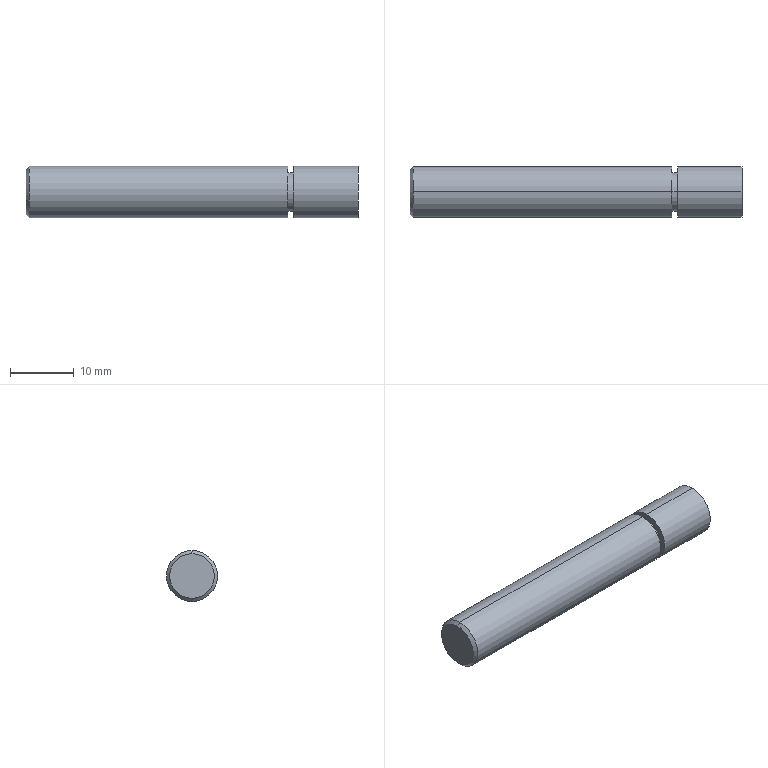Part | STEP file | 0246_222_Pin | 1 solid | 15 faces | box 52 x 8 x 8 mm | volume 2505 mm3 | cylinder 8 | plane 5 | cone 2 | commonest cylinder face diameters 8 x4 3.3 x2 6 x2
STEP:
#1=CARTESIAN_POINT('',(0.,0.,0.));
#2=DIRECTION('',(0.,0.,1.));
#3=DIRECTION('',(1.,0.,0.));
#4=AXIS2_PLACEMENT_3D('',#1,#2,#3);
#5=CARTESIAN_POINT('',(-41.,0.,3.5));
#6=VERTEX_POINT('',#5);
#7=CARTESIAN_POINT('',(-41.,0.,-3.5));
#8=VERTEX_POINT('',#7);
#9=CARTESIAN_POINT('',(-41.,0.,0.));
#10=DIRECTION('',(-1.,0.,0.));
#11=DIRECTION('',(0.,0.,-1.));
#12=AXIS2_PLACEMENT_3D('',#9,#10,#11);
#13=CIRCLE('',#12,3.5);
#14=CARTESIAN_POINT('',(-41.,0.,0.));
#15=DIRECTION('',(1.,0.,0.));
#16=DIRECTION('',(0.,0.,-1.));
#17=AXIS2_PLACEMENT_3D('',#14,#15,#16);
#18=CONICAL_SURFACE('',#17,3.5,0.7854);
#19=CARTESIAN_POINT('',(6.283,0.));
#20=DIRECTION('',(-1.,0.));
#21=VECTOR('',#20,1.);
#22=LINE('',#19,#21);
#23=(GEOMETRIC_REPRESENTATION_CONTEXT(2)PARAMETRIC_REPRESENTATION_CONTEXT()REPRESENTATION_CONTEXT('',''));
#24=DEFINITIONAL_REPRESENTATION('',(#22),#23);
#25=PCURVE('',#18,#24);
#26=CARTESIAN_POINT('',(-41.,-4.,0.));
#27=DIRECTION('',(1.,0.,0.));
#28=DIRECTION('',(0.,0.,-1.));
#29=AXIS2_PLACEMENT_3D('',#26,#27,#28);
#30=PLANE('',#29);
#31=CARTESIAN_POINT('',(3.5,4.));
#32=CARTESIAN_POINT('',(3.5,-2.062));
#33=CARTESIAN_POINT('',(-1.75,0.9689));
#34=CARTESIAN_POINT('',(-7.,4.));
#35=CARTESIAN_POINT('',(-1.75,7.031));
#36=CARTESIAN_POINT('',(3.5,10.062));
#37=CARTESIAN_POINT('',(3.5,4.));
#38=(BOUNDED_CURVE()B_SPLINE_CURVE(2,(#31,#32,#33,#34,#35,#36,#37),.UNSPECIFIED.,.T.,.F.)B_SPLINE_CURVE_WITH_KNOTS((1,2,2,2,2,1),(-2.094,0.,2.094,4.189,6.283,8.378),.UNSPECIFIED.)CURVE()GEOMETRIC_REPRESENTATION_ITEM()RATIONAL_B_SPLINE_CURVE((1.,0.5,1.,0.5,1.,0.5,1.))REPRESENTATION_ITEM(''));
#39=(GEOMETRIC_REPRESENTATION_CONTEXT(2)PARAMETRIC_REPRESENTATION_CONTEXT()REPRESENTATION_CONTEXT('',''));
#40=DEFINITIONAL_REPRESENTATION('',(#38),#39);
#41=PCURVE('',#30,#40);
#42=SURFACE_CURVE('',#13,(#25,#41),.PCURVE_S1.);
#43=EDGE_CURVE('',#6,#8,#42,.T.);
#44=ORIENTED_EDGE('',*,*,#43,.F.);
#45=CARTESIAN_POINT('',(-40.5,0.,4.));
#46=VERTEX_POINT('',#45);
#47=CARTESIAN_POINT('',(-41.,0.,3.5));
#48=DIRECTION('',(0.7071,0.,0.7071));
#49=VECTOR('',#48,1.);
#50=LINE('',#47,#49);
#51=CARTESIAN_POINT('',(3.142,0.));
#52=DIRECTION('',(0.,1.));
#53=VECTOR('',#52,1.);
#54=LINE('',#51,#53);
#55=(GEOMETRIC_REPRESENTATION_CONTEXT(2)PARAMETRIC_REPRESENTATION_CONTEXT()REPRESENTATION_CONTEXT('',''));
#56=DEFINITIONAL_REPRESENTATION('',(#54),#55);
#57=PCURVE('',#18,#56);
#58=CARTESIAN_POINT('',(-41.,0.,0.));
#59=DIRECTION('',(1.,0.,0.));
#60=DIRECTION('',(0.,0.,-1.));
#61=AXIS2_PLACEMENT_3D('',#58,#59,#60);
#62=CONICAL_SURFACE('',#61,3.5,0.7854);
#63=CARTESIAN_POINT('',(3.142,0.));
#64=DIRECTION('',(0.,1.));
#65=VECTOR('',#64,1.);
#66=LINE('',#63,#65);
#67=(GEOMETRIC_REPRESENTATION_CONTEXT(2)PARAMETRIC_REPRESENTATION_CONTEXT()REPRESENTATION_CONTEXT('',''));
#68=DEFINITIONAL_REPRESENTATION('',(#66),#67);
#69=PCURVE('',#62,#68);
#70=SURFACE_CURVE('',#50,(#57,#69),.PCURVE_S1.);
#71=EDGE_CURVE('',#6,#46,#70,.T.);
#72=ORIENTED_EDGE('',*,*,#71,.T.);
#73=CARTESIAN_POINT('',(-40.5,0.,-4.));
#74=VERTEX_POINT('',#73);
#75=CARTESIAN_POINT('',(-40.5,0.,0.));
#76=DIRECTION('',(1.,0.,0.));
#77=DIRECTION('',(0.,0.,-1.));
#78=AXIS2_PLACEMENT_3D('',#75,#76,#77);
#79=CIRCLE('',#78,4.);
#80=CARTESIAN_POINT('',(0.,0.5));
#81=DIRECTION('',(1.,0.));
#82=VECTOR('',#81,1.);
#83=LINE('',#80,#82);
#84=(GEOMETRIC_REPRESENTATION_CONTEXT(2)PARAMETRIC_REPRESENTATION_CONTEXT()REPRESENTATION_CONTEXT('',''));
#85=DEFINITIONAL_REPRESENTATION('',(#83),#84);
#86=PCURVE('',#18,#85);
#87=CARTESIAN_POINT('',(-41.,0.,0.));
#88=DIRECTION('',(-1.,0.,0.));
#89=DIRECTION('',(0.,0.,1.));
#90=AXIS2_PLACEMENT_3D('',#87,#88,#89);
#91=CYLINDRICAL_SURFACE('',#90,4.);
#92=CARTESIAN_POINT('',(3.142,-0.5));
#93=DIRECTION('',(-1.,0.));
#94=VECTOR('',#93,1.);
#95=LINE('',#92,#94);
#96=(GEOMETRIC_REPRESENTATION_CONTEXT(2)PARAMETRIC_REPRESENTATION_CONTEXT()REPRESENTATION_CONTEXT('',''));
#97=DEFINITIONAL_REPRESENTATION('',(#95),#96);
#98=PCURVE('',#91,#97);
#99=SURFACE_CURVE('',#79,(#86,#98),.PCURVE_S1.);
#100=EDGE_CURVE('',#74,#46,#99,.T.);
#101=ORIENTED_EDGE('',*,*,#100,.F.);
#102=CARTESIAN_POINT('',(-41.,0.,-3.5));
#103=DIRECTION('',(0.7071,0.,-0.7071));
#104=VECTOR('',#103,1.);
#105=LINE('',#102,#104);
#106=CARTESIAN_POINT('',(0.,0.));
#107=DIRECTION('',(0.,1.));
#108=VECTOR('',#107,1.);
#109=LINE('',#106,#108);
#110=(GEOMETRIC_REPRESENTATION_CONTEXT(2)PARAMETRIC_REPRESENTATION_CONTEXT()REPRESENTATION_CONTEXT('',''));
#111=DEFINITIONAL_REPRESENTATION('',(#109),#110);
#112=PCURVE('',#18,#111);
#113=CARTESIAN_POINT('',(6.283,0.));
#114=DIRECTION('',(0.,1.));
#115=VECTOR('',#114,1.);
#116=LINE('',#113,#115);
#117=(GEOMETRIC_REPRESENTATION_CONTEXT(2)PARAMETRIC_REPRESENTATION_CONTEXT()REPRESENTATION_CONTEXT('',''));
#118=DEFINITIONAL_REPRESENTATION('',(#116),#117);
#119=PCURVE('',#62,#118);
#120=SURFACE_CURVE('',#105,(#112,#119),.PCURVE_S1.);
#121=EDGE_CURVE('',#8,#74,#120,.T.);
#122=ORIENTED_EDGE('',*,*,#121,.F.);
#123=EDGE_LOOP('',(#44,#72,#101,#122));
#124=FACE_BOUND('',#123,.T.);
#125=ADVANCED_FACE('',(#124),#18,.T.);
#126=CARTESIAN_POINT('',(0.9,0.,-1.65));
#127=VERTEX_POINT('',#126);
#128=CARTESIAN_POINT('',(11.,0.,-1.65));
#129=VERTEX_POINT('',#128);
#130=CARTESIAN_POINT('',(11.,0.,-1.65));
#131=DIRECTION('',(1.,0.,0.));
#132=VECTOR('',#131,1.);
#133=LINE('',#130,#132);
#134=CARTESIAN_POINT('',(11.,0.,0.));
#135=DIRECTION('',(1.,0.,0.));
#136=DIRECTION('',(0.,0.,-1.));
#137=AXIS2_PLACEMENT_3D('',#134,#135,#136);
#138=CYLINDRICAL_SURFACE('',#137,1.65);
#139=CARTESIAN_POINT('',(6.283,0.));
#140=DIRECTION('',(0.,1.));
#141=VECTOR('',#140,1.);
#142=LINE('',#139,#141);
#143=(GEOMETRIC_REPRESENTATION_CONTEXT(2)PARAMETRIC_REPRESENTATION_CONTEXT()REPRESENTATION_CONTEXT('',''));
#144=DEFINITIONAL_REPRESENTATION('',(#142),#143);
#145=PCURVE('',#138,#144);
#146=CARTESIAN_POINT('',(11.,0.,0.));
#147=DIRECTION('',(1.,0.,0.));
#148=DIRECTION('',(0.,0.,-1.));
#149=AXIS2_PLACEMENT_3D('',#146,#147,#148);
#150=CYLINDRICAL_SURFACE('',#149,1.65);
#151=CARTESIAN_POINT('',(0.,0.));
#152=DIRECTION('',(0.,1.));
#153=VECTOR('',#152,1.);
#154=LINE('',#151,#153);
#155=(GEOMETRIC_REPRESENTATION_CONTEXT(2)PARAMETRIC_REPRESENTATION_CONTEXT()REPRESENTATION_CONTEXT('',''));
#156=DEFINITIONAL_REPRESENTATION('',(#154),#155);
#157=PCURVE('',#150,#156);
#158=SURFACE_CURVE('',#133,(#145,#157),.PCURVE_S1.);
#159=EDGE_CURVE('',#127,#129,#158,.T.);
#160=ORIENTED_EDGE('',*,*,#159,.T.);
#161=CARTESIAN_POINT('',(11.,0.,1.65));
#162=VERTEX_POINT('',#161);
#163=CARTESIAN_POINT('',(11.,0.,0.));
#164=DIRECTION('',(1.,0.,0.));
#165=DIRECTION('',(0.,0.,-1.));
#166=AXIS2_PLACEMENT_3D('',#163,#164,#165);
#167=CIRCLE('',#166,1.65);
#168=CARTESIAN_POINT('',(0.,0.));
#169=DIRECTION('',(1.,0.));
#170=VECTOR('',#169,1.);
#171=LINE('',#168,#170);
#172=(GEOMETRIC_REPRESENTATION_CONTEXT(2)PARAMETRIC_REPRESENTATION_CONTEXT()REPRESENTATION_CONTEXT('',''));
#173=DEFINITIONAL_REPRESENTATION('',(#171),#172);
#174=PCURVE('',#138,#173);
#175=CARTESIAN_POINT('',(11.,-4.,0.));
#176=DIRECTION('',(-1.,0.,0.));
#177=DIRECTION('',(0.,0.,1.));
#178=AXIS2_PLACEMENT_3D('',#175,#176,#177);
#179=PLANE('',#178);
#180=CARTESIAN_POINT('',(-1.65,4.));
#181=CARTESIAN_POINT('',(-1.65,6.858));
#182=CARTESIAN_POINT('',(0.825,5.429));
#183=CARTESIAN_POINT('',(3.3,4.));
#184=CARTESIAN_POINT('',(0.825,2.571));
#185=CARTESIAN_POINT('',(-1.65,1.142));
#186=CARTESIAN_POINT('',(-1.65,4.));
#187=(BOUNDED_CURVE()B_SPLINE_CURVE(2,(#180,#181,#182,#183,#184,#185,#186),.UNSPECIFIED.,.T.,.F.)B_SPLINE_CURVE_WITH_KNOTS((1,2,2,2,2,1),(-2.094,0.,2.094,4.189,6.283,8.378),.UNSPECIFIED.)CURVE()GEOMETRIC_REPRESENTATION_ITEM()RATIONAL_B_SPLINE_CURVE((1.,0.5,1.,0.5,1.,0.5,1.))REPRESENTATION_ITEM(''));
#188=(GEOMETRIC_REPRESENTATION_CONTEXT(2)PARAMETRIC_REPRESENTATION_CONTEXT()REPRESENTATION_CONTEXT('',''));
#189=DEFINITIONAL_REPRESENTATION('',(#187),#188);
#190=PCURVE('',#179,#189);
#191=SURFACE_CURVE('',#167,(#174,#190),.PCURVE_S1.);
#192=EDGE_CURVE('',#162,#129,#191,.T.);
#193=ORIENTED_EDGE('',*,*,#192,.F.);
#194=CARTESIAN_POINT('',(0.9,0.,1.65));
#195=VERTEX_POINT('',#194);
#196=CARTESIAN_POINT('',(11.,0.,1.65));
#197=DIRECTION('',(1.,0.,0.));
#198=VECTOR('',#197,1.);
#199=LINE('',#196,#198);
#200=CARTESIAN_POINT('',(3.142,0.));
#201=DIRECTION('',(0.,1.));
#202=VECTOR('',#201,1.);
#203=LINE('',#200,#202);
#204=(GEOMETRIC_REPRESENTATION_CONTEXT(2)PARAMETRIC_REPRESENTATION_CONTEXT()REPRESENTATION_CONTEXT('',''));
#205=DEFINITIONAL_REPRESENTATION('',(#203),#204);
#206=PCURVE('',#138,#205);
#207=CARTESIAN_POINT('',(3.142,0.));
#208=DIRECTION('',(0.,1.));
#209=VECTOR('',#208,1.);
#210=LINE('',#207,#209);
#211=(GEOMETRIC_REPRESENTATION_CONTEXT(2)PARAMETRIC_REPRESENTATION_CONTEXT()REPRESENTATION_CONTEXT('',''));
#212=DEFINITIONAL_REPRESENTATION('',(#210),#211);
#213=PCURVE('',#150,#212);
#214=SURFACE_CURVE('',#199,(#206,#213),.PCURVE_S1.);
#215=EDGE_CURVE('',#195,#162,#214,.T.);
#216=ORIENTED_EDGE('',*,*,#215,.F.);
#217=CARTESIAN_POINT('',(0.9,0.,0.));
#218=DIRECTION('',(1.,0.,0.));
#219=DIRECTION('',(0.,0.,-1.));
#220=AXIS2_PLACEMENT_3D('',#217,#218,#219);
#221=CIRCLE('',#220,1.65);
#222=CARTESIAN_POINT('',(0.,-10.1));
#223=DIRECTION('',(1.,0.));
#224=VECTOR('',#223,1.);
#225=LINE('',#222,#224);
#226=(GEOMETRIC_REPRESENTATION_CONTEXT(2)PARAMETRIC_REPRESENTATION_CONTEXT()REPRESENTATION_CONTEXT('',''));
#227=DEFINITIONAL_REPRESENTATION('',(#225),#226);
#228=PCURVE('',#138,#227);
#229=CARTESIAN_POINT('',(0.9,0.,0.));
#230=DIRECTION('',(-1.,0.,0.));
#231=DIRECTION('',(0.,0.,1.));
#232=AXIS2_PLACEMENT_3D('',#229,#230,#231);
#233=PLANE('',#232);
#234=CARTESIAN_POINT('',(-1.65,0.));
#235=CARTESIAN_POINT('',(-1.65,2.858));
#236=CARTESIAN_POINT('',(0.825,1.429));
#237=CARTESIAN_POINT('',(3.3,0.));
#238=CARTESIAN_POINT('',(0.825,-1.429));
#239=CARTESIAN_POINT('',(-1.65,-2.858));
#240=CARTESIAN_POINT('',(-1.65,0.));
#241=(BOUNDED_CURVE()B_SPLINE_CURVE(2,(#234,#235,#236,#237,#238,#239,#240),.UNSPECIFIED.,.T.,.F.)B_SPLINE_CURVE_WITH_KNOTS((1,2,2,2,2,1),(-2.094,0.,2.094,4.189,6.283,8.378),.UNSPECIFIED.)CURVE()GEOMETRIC_REPRESENTATION_ITEM()RATIONAL_B_SPLINE_CURVE((1.,0.5,1.,0.5,1.,0.5,1.))REPRESENTATION_ITEM(''));
#242=(GEOMETRIC_REPRESENTATION_CONTEXT(2)PARAMETRIC_REPRESENTATION_CONTEXT()REPRESENTATION_CONTEXT('',''));
#243=DEFINITIONAL_REPRESENTATION('',(#241),#242);
#244=PCURVE('',#233,#243);
#245=SURFACE_CURVE('',#221,(#228,#244),.PCURVE_S1.);
#246=EDGE_CURVE('',#195,#127,#245,.T.);
#247=ORIENTED_EDGE('',*,*,#246,.T.);
#248=EDGE_LOOP('',(#160,#193,#216,#247));
#249=FACE_BOUND('',#248,.F.);
#250=ADVANCED_FACE('',(#249),#138,.F.);
#251=CARTESIAN_POINT('',(11.,0.,4.));
#252=VERTEX_POINT('',#251);
#253=CARTESIAN_POINT('',(11.,0.,-4.));
#254=VERTEX_POINT('',#253);
#255=CARTESIAN_POINT('',(11.,0.,0.));
#256=DIRECTION('',(-1.,0.,0.));
#257=DIRECTION('',(0.,0.,1.));
#258=AXIS2_PLACEMENT_3D('',#255,#256,#257);
#259=CIRCLE('',#258,4.);
#260=CARTESIAN_POINT('',(-41.,0.,0.));
#261=DIRECTION('',(-1.,0.,0.));
#262=DIRECTION('',(0.,0.,1.));
#263=AXIS2_PLACEMENT_3D('',#260,#261,#262);
#264=CYLINDRICAL_SURFACE('',#263,4.);
#265=CARTESIAN_POINT('',(0.,-52.));
#266=DIRECTION('',(1.,0.));
#267=VECTOR('',#266,1.);
#268=LINE('',#265,#267);
#269=(GEOMETRIC_REPRESENTATION_CONTEXT(2)PARAMETRIC_REPRESENTATION_CONTEXT()REPRESENTATION_CONTEXT('',''));
#270=DEFINITIONAL_REPRESENTATION('',(#268),#269);
#271=PCURVE('',#264,#270);
#272=CARTESIAN_POINT('',(0.,4.));
#273=DIRECTION('',(1.,0.));
#274=AXIS2_PLACEMENT_2D('',#272,#273);
#275=CIRCLE('',#274,4.);
#276=(GEOMETRIC_REPRESENTATION_CONTEXT(2)PARAMETRIC_REPRESENTATION_CONTEXT()REPRESENTATION_CONTEXT('',''));
#277=DEFINITIONAL_REPRESENTATION('',(#275),#276);
#278=PCURVE('',#179,#277);
#279=SURFACE_CURVE('',#259,(#271,#278),.PCURVE_S1.);
#280=EDGE_CURVE('',#252,#254,#279,.T.);
#281=ORIENTED_EDGE('',*,*,#280,.T.);
#282=CARTESIAN_POINT('',(0.9,0.,-4.));
#283=VERTEX_POINT('',#282);
#284=CARTESIAN_POINT('',(-41.,0.,-4.));
#285=DIRECTION('',(-1.,0.,0.));
#286=VECTOR('',#285,1.);
#287=LINE('',#284,#286);
#288=CARTESIAN_POINT('',(3.142,0.));
#289=DIRECTION('',(0.,1.));
#290=VECTOR('',#289,1.);
#291=LINE('',#288,#290);
#292=(GEOMETRIC_REPRESENTATION_CONTEXT(2)PARAMETRIC_REPRESENTATION_CONTEXT()REPRESENTATION_CONTEXT('',''));
#293=DEFINITIONAL_REPRESENTATION('',(#291),#292);
#294=PCURVE('',#264,#293);
#295=CARTESIAN_POINT('',(-41.,0.,0.));
#296=DIRECTION('',(-1.,0.,0.));
#297=DIRECTION('',(0.,0.,1.));
#298=AXIS2_PLACEMENT_3D('',#295,#296,#297);
#299=CYLINDRICAL_SURFACE('',#298,4.);
#300=CARTESIAN_POINT('',(3.142,0.));
#301=DIRECTION('',(0.,1.));
#302=VECTOR('',#301,1.);
#303=LINE('',#300,#302);
#304=(GEOMETRIC_REPRESENTATION_CONTEXT(2)PARAMETRIC_REPRESENTATION_CONTEXT()REPRESENTATION_CONTEXT('',''));
#305=DEFINITIONAL_REPRESENTATION('',(#303),#304);
#306=PCURVE('',#299,#305);
#307=SURFACE_CURVE('',#287,(#294,#306),.PCURVE_S1.);
#308=EDGE_CURVE('',#254,#283,#307,.T.);
#309=ORIENTED_EDGE('',*,*,#308,.T.);
#310=CARTESIAN_POINT('',(0.9,0.,4.));
#311=VERTEX_POINT('',#310);
#312=CARTESIAN_POINT('',(0.9,0.,0.));
#313=DIRECTION('',(-1.,0.,0.));
#314=DIRECTION('',(0.,0.,1.));
#315=AXIS2_PLACEMENT_3D('',#312,#313,#314);
#316=CIRCLE('',#315,4.);
#317=CARTESIAN_POINT('',(0.,-41.9));
#318=DIRECTION('',(1.,0.));
#319=VECTOR('',#318,1.);
#320=LINE('',#317,#319);
#321=(GEOMETRIC_REPRESENTATION_CONTEXT(2)PARAMETRIC_REPRESENTATION_CONTEXT()REPRESENTATION_CONTEXT('',''));
#322=DEFINITIONAL_REPRESENTATION('',(#320),#321);
#323=PCURVE('',#264,#322);
#324=CARTESIAN_POINT('',(0.9,-3.,0.));
#325=DIRECTION('',(1.,0.,0.));
#326=DIRECTION('',(0.,0.,-1.));
#327=AXIS2_PLACEMENT_3D('',#324,#325,#326);
#328=PLANE('',#327);
#329=CARTESIAN_POINT('',(-4.,3.));
#330=CARTESIAN_POINT('',(-4.,9.928));
#331=CARTESIAN_POINT('',(2.,6.464));
#332=CARTESIAN_POINT('',(8.,3.));
#333=CARTESIAN_POINT('',(2.,-0.4641));
#334=CARTESIAN_POINT('',(-4.,-3.928));
#335=CARTESIAN_POINT('',(-4.,3.));
#336=(BOUNDED_CURVE()B_SPLINE_CURVE(2,(#329,#330,#331,#332,#333,#334,#335),.UNSPECIFIED.,.T.,.F.)B_SPLINE_CURVE_WITH_KNOTS((1,2,2,2,2,1),(-2.094,0.,2.094,4.189,6.283,8.378),.UNSPECIFIED.)CURVE()GEOMETRIC_REPRESENTATION_ITEM()RATIONAL_B_SPLINE_CURVE((1.,0.5,1.,0.5,1.,0.5,1.))REPRESENTATION_ITEM(''));
#337=(GEOMETRIC_REPRESENTATION_CONTEXT(2)PARAMETRIC_REPRESENTATION_CONTEXT()REPRESENTATION_CONTEXT('',''));
#338=DEFINITIONAL_REPRESENTATION('',(#336),#337);
#339=PCURVE('',#328,#338);
#340=SURFACE_CURVE('',#316,(#323,#339),.PCURVE_S1.);
#341=EDGE_CURVE('',#311,#283,#340,.T.);
#342=ORIENTED_EDGE('',*,*,#341,.F.);
#343=CARTESIAN_POINT('',(-41.,0.,4.));
#344=DIRECTION('',(-1.,0.,0.));
#345=VECTOR('',#344,1.);
#346=LINE('',#343,#345);
#347=CARTESIAN_POINT('',(0.,0.));
#348=DIRECTION('',(0.,1.));
#349=VECTOR('',#348,1.);
#350=LINE('',#347,#349);
#351=(GEOMETRIC_REPRESENTATION_CONTEXT(2)PARAMETRIC_REPRESENTATION_CONTEXT()REPRESENTATION_CONTEXT('',''));
#352=DEFINITIONAL_REPRESENTATION('',(#350),#351);
#353=PCURVE('',#264,#352);
#354=CARTESIAN_POINT('',(6.283,0.));
#355=DIRECTION('',(0.,1.));
#356=VECTOR('',#355,1.);
#357=LINE('',#354,#356);
#358=(GEOMETRIC_REPRESENTATION_CONTEXT(2)PARAMETRIC_REPRESENTATION_CONTEXT()REPRESENTATION_CONTEXT('',''));
#359=DEFINITIONAL_REPRESENTATION('',(#357),#358);
#360=PCURVE('',#299,#359);
#361=SURFACE_CURVE('',#346,(#353,#360),.PCURVE_S1.);
#362=EDGE_CURVE('',#252,#311,#361,.T.);
#363=ORIENTED_EDGE('',*,*,#362,.F.);
#364=EDGE_LOOP('',(#281,#309,#342,#363));
#365=FACE_BOUND('',#364,.T.);
#366=ADVANCED_FACE('',(#365),#264,.T.);
#367=CARTESIAN_POINT('',(0.9,0.,3.));
#368=VERTEX_POINT('',#367);
#369=CARTESIAN_POINT('',(0.9,0.,-3.));
#370=VERTEX_POINT('',#369);
#371=CARTESIAN_POINT('',(0.9,0.,0.));
#372=DIRECTION('',(-1.,0.,0.));
#373=DIRECTION('',(0.,0.,1.));
#374=AXIS2_PLACEMENT_3D('',#371,#372,#373);
#375=CIRCLE('',#374,3.);
#376=CARTESIAN_POINT('',(-41.,0.,0.));
#377=DIRECTION('',(-1.,0.,0.));
#378=DIRECTION('',(0.,0.,1.));
#379=AXIS2_PLACEMENT_3D('',#376,#377,#378);
#380=CYLINDRICAL_SURFACE('',#379,3.);
#381=CARTESIAN_POINT('',(0.,-41.9));
#382=DIRECTION('',(1.,0.));
#383=VECTOR('',#382,1.);
#384=LINE('',#381,#383);
#385=(GEOMETRIC_REPRESENTATION_CONTEXT(2)PARAMETRIC_REPRESENTATION_CONTEXT()REPRESENTATION_CONTEXT('',''));
#386=DEFINITIONAL_REPRESENTATION('',(#384),#385);
#387=PCURVE('',#380,#386);
#388=CARTESIAN_POINT('',(-3.,3.));
#389=CARTESIAN_POINT('',(-3.,8.196));
#390=CARTESIAN_POINT('',(1.5,5.598));
#391=CARTESIAN_POINT('',(6.,3.));
#392=CARTESIAN_POINT('',(1.5,0.4019));
#393=CARTESIAN_POINT('',(-3.,-2.196));
#394=CARTESIAN_POINT('',(-3.,3.));
#395=(BOUNDED_CURVE()B_SPLINE_CURVE(2,(#388,#389,#390,#391,#392,#393,#394),.UNSPECIFIED.,.T.,.F.)B_SPLINE_CURVE_WITH_KNOTS((1,2,2,2,2,1),(-2.094,0.,2.094,4.189,6.283,8.378),.UNSPECIFIED.)CURVE()GEOMETRIC_REPRESENTATION_ITEM()RATIONAL_B_SPLINE_CURVE((1.,0.5,1.,0.5,1.,0.5,1.))REPRESENTATION_ITEM(''));
#396=(GEOMETRIC_REPRESENTATION_CONTEXT(2)PARAMETRIC_REPRESENTATION_CONTEXT()REPRESENTATION_CONTEXT('',''));
#397=DEFINITIONAL_REPRESENTATION('',(#395),#396);
#398=PCURVE('',#328,#397);
#399=SURFACE_CURVE('',#375,(#387,#398),.PCURVE_S1.);
#400=EDGE_CURVE('',#368,#370,#399,.T.);
#401=ORIENTED_EDGE('',*,*,#400,.T.);
#402=CARTESIAN_POINT('',(0.,0.,-3.));
#403=VERTEX_POINT('',#402);
#404=CARTESIAN_POINT('',(-41.,0.,-3.));
#405=DIRECTION('',(-1.,0.,0.));
#406=VECTOR('',#405,1.);
#407=LINE('',#404,#406);
#408=CARTESIAN_POINT('',(3.142,0.));
#409=DIRECTION('',(0.,1.));
#410=VECTOR('',#409,1.);
#411=LINE('',#408,#410);
#412=(GEOMETRIC_REPRESENTATION_CONTEXT(2)PARAMETRIC_REPRESENTATION_CONTEXT()REPRESENTATION_CONTEXT('',''));
#413=DEFINITIONAL_REPRESENTATION('',(#411),#412);
#414=PCURVE('',#380,#413);
#415=CARTESIAN_POINT('',(-41.,0.,0.));
#416=DIRECTION('',(-1.,0.,0.));
#417=DIRECTION('',(0.,0.,1.));
#418=AXIS2_PLACEMENT_3D('',#415,#416,#417);
#419=CYLINDRICAL_SURFACE('',#418,3.);
#420=CARTESIAN_POINT('',(3.142,0.));
#421=DIRECTION('',(0.,1.));
#422=VECTOR('',#421,1.);
#423=LINE('',#420,#422);
#424=(GEOMETRIC_REPRESENTATION_CONTEXT(2)PARAMETRIC_REPRESENTATION_CONTEXT()REPRESENTATION_CONTEXT('',''));
#425=DEFINITIONAL_REPRESENTATION('',(#423),#424);
#426=PCURVE('',#419,#425);
#427=SURFACE_CURVE('',#407,(#414,#426),.PCURVE_S1.);
#428=EDGE_CURVE('',#370,#403,#427,.T.);
#429=ORIENTED_EDGE('',*,*,#428,.T.);
#430=CARTESIAN_POINT('',(0.,0.,3.));
#431=VERTEX_POINT('',#430);
#432=CARTESIAN_POINT('',(0.,0.,0.));
#433=DIRECTION('',(-1.,0.,0.));
#434=DIRECTION('',(0.,0.,1.));
#435=AXIS2_PLACEMENT_3D('',#432,#433,#434);
#436=CIRCLE('',#435,3.);
#437=CARTESIAN_POINT('',(0.,-41.));
#438=DIRECTION('',(1.,0.));
#439=VECTOR('',#438,1.);
#440=LINE('',#437,#439);
#441=(GEOMETRIC_REPRESENTATION_CONTEXT(2)PARAMETRIC_REPRESENTATION_CONTEXT()REPRESENTATION_CONTEXT('',''));
#442=DEFINITIONAL_REPRESENTATION('',(#440),#441);
#443=PCURVE('',#380,#442);
#444=CARTESIAN_POINT('',(0.,-3.,0.));
#445=DIRECTION('',(-1.,0.,0.));
#446=DIRECTION('',(0.,0.,1.));
#447=AXIS2_PLACEMENT_3D('',#444,#445,#446);
#448=PLANE('',#447);
#449=CARTESIAN_POINT('',(0.,3.));
#450=DIRECTION('',(1.,0.));
#451=AXIS2_PLACEMENT_2D('',#449,#450);
#452=CIRCLE('',#451,3.);
#453=(GEOMETRIC_REPRESENTATION_CONTEXT(2)PARAMETRIC_REPRESENTATION_CONTEXT()REPRESENTATION_CONTEXT('',''));
#454=DEFINITIONAL_REPRESENTATION('',(#452),#453);
#455=PCURVE('',#448,#454);
#456=SURFACE_CURVE('',#436,(#443,#455),.PCURVE_S1.);
#457=EDGE_CURVE('',#431,#403,#456,.T.);
#458=ORIENTED_EDGE('',*,*,#457,.F.);
#459=CARTESIAN_POINT('',(-41.,0.,3.));
#460=DIRECTION('',(-1.,0.,0.));
#461=VECTOR('',#460,1.);
#462=LINE('',#459,#461);
#463=CARTESIAN_POINT('',(0.,0.));
#464=DIRECTION('',(0.,1.));
#465=VECTOR('',#464,1.);
#466=LINE('',#463,#465);
#467=(GEOMETRIC_REPRESENTATION_CONTEXT(2)PARAMETRIC_REPRESENTATION_CONTEXT()REPRESENTATION_CONTEXT('',''));
#468=DEFINITIONAL_REPRESENTATION('',(#466),#467);
#469=PCURVE('',#380,#468);
#470=CARTESIAN_POINT('',(6.283,0.));
#471=DIRECTION('',(0.,1.));
#472=VECTOR('',#471,1.);
#473=LINE('',#470,#472);
#474=(GEOMETRIC_REPRESENTATION_CONTEXT(2)PARAMETRIC_REPRESENTATION_CONTEXT()REPRESENTATION_CONTEXT('',''));
#475=DEFINITIONAL_REPRESENTATION('',(#473),#474);
#476=PCURVE('',#419,#475);
#477=SURFACE_CURVE('',#462,(#469,#476),.PCURVE_S1.);
#478=EDGE_CURVE('',#368,#431,#477,.T.);
#479=ORIENTED_EDGE('',*,*,#478,.F.);
#480=EDGE_LOOP('',(#401,#429,#458,#479));
#481=FACE_BOUND('',#480,.T.);
#482=ADVANCED_FACE('',(#481),#380,.T.);
#483=CARTESIAN_POINT('',(0.,0.,4.));
#484=VERTEX_POINT('',#483);
#485=CARTESIAN_POINT('',(0.,0.,-4.));
#486=VERTEX_POINT('',#485);
#487=CARTESIAN_POINT('',(0.,0.,0.));
#488=DIRECTION('',(-1.,0.,0.));
#489=DIRECTION('',(0.,0.,1.));
#490=AXIS2_PLACEMENT_3D('',#487,#488,#489);
#491=CIRCLE('',#490,4.);
#492=CARTESIAN_POINT('',(0.,-41.));
#493=DIRECTION('',(1.,0.));
#494=VECTOR('',#493,1.);
#495=LINE('',#492,#494);
#496=(GEOMETRIC_REPRESENTATION_CONTEXT(2)PARAMETRIC_REPRESENTATION_CONTEXT()REPRESENTATION_CONTEXT('',''));
#497=DEFINITIONAL_REPRESENTATION('',(#495),#496);
#498=PCURVE('',#91,#497);
#499=CARTESIAN_POINT('',(0.,3.));
#500=DIRECTION('',(1.,0.));
#501=AXIS2_PLACEMENT_2D('',#499,#500);
#502=CIRCLE('',#501,4.);
#503=(GEOMETRIC_REPRESENTATION_CONTEXT(2)PARAMETRIC_REPRESENTATION_CONTEXT()REPRESENTATION_CONTEXT('',''));
#504=DEFINITIONAL_REPRESENTATION('',(#502),#503);
#505=PCURVE('',#448,#504);
#506=SURFACE_CURVE('',#491,(#498,#505),.PCURVE_S1.);
#507=EDGE_CURVE('',#484,#486,#506,.T.);
#508=ORIENTED_EDGE('',*,*,#507,.T.);
#509=CARTESIAN_POINT('',(-41.,0.,-4.));
#510=DIRECTION('',(-1.,0.,0.));
#511=VECTOR('',#510,1.);
#512=LINE('',#509,#511);
#513=CARTESIAN_POINT('',(3.142,0.));
#514=DIRECTION('',(0.,1.));
#515=VECTOR('',#514,1.);
#516=LINE('',#513,#515);
#517=(GEOMETRIC_REPRESENTATION_CONTEXT(2)PARAMETRIC_REPRESENTATION_CONTEXT()REPRESENTATION_CONTEXT('',''));
#518=DEFINITIONAL_REPRESENTATION('',(#516),#517);
#519=PCURVE('',#91,#518);
#520=CARTESIAN_POINT('',(-41.,0.,0.));
#521=DIRECTION('',(-1.,0.,0.));
#522=DIRECTION('',(0.,0.,1.));
#523=AXIS2_PLACEMENT_3D('',#520,#521,#522);
#524=CYLINDRICAL_SURFACE('',#523,4.);
#525=CARTESIAN_POINT('',(3.142,0.));
#526=DIRECTION('',(0.,1.));
#527=VECTOR('',#526,1.);
#528=LINE('',#525,#527);
#529=(GEOMETRIC_REPRESENTATION_CONTEXT(2)PARAMETRIC_REPRESENTATION_CONTEXT()REPRESENTATION_CONTEXT('',''));
#530=DEFINITIONAL_REPRESENTATION('',(#528),#529);
#531=PCURVE('',#524,#530);
#532=SURFACE_CURVE('',#512,(#519,#531),.PCURVE_S1.);
#533=EDGE_CURVE('',#486,#74,#532,.T.);
#534=ORIENTED_EDGE('',*,*,#533,.T.);
#535=ORIENTED_EDGE('',*,*,#100,.T.);
#536=CARTESIAN_POINT('',(-41.,0.,4.));
#537=DIRECTION('',(-1.,0.,0.));
#538=VECTOR('',#537,1.);
#539=LINE('',#536,#538);
#540=CARTESIAN_POINT('',(0.,0.));
#541=DIRECTION('',(0.,1.));
#542=VECTOR('',#541,1.);
#543=LINE('',#540,#542);
#544=(GEOMETRIC_REPRESENTATION_CONTEXT(2)PARAMETRIC_REPRESENTATION_CONTEXT()REPRESENTATION_CONTEXT('',''));
#545=DEFINITIONAL_REPRESENTATION('',(#543),#544);
#546=PCURVE('',#91,#545);
#547=CARTESIAN_POINT('',(6.283,0.));
#548=DIRECTION('',(0.,1.));
#549=VECTOR('',#548,1.);
#550=LINE('',#547,#549);
#551=(GEOMETRIC_REPRESENTATION_CONTEXT(2)PARAMETRIC_REPRESENTATION_CONTEXT()REPRESENTATION_CONTEXT('',''));
#552=DEFINITIONAL_REPRESENTATION('',(#550),#551);
#553=PCURVE('',#524,#552);
#554=SURFACE_CURVE('',#539,(#546,#553),.PCURVE_S1.);
#555=EDGE_CURVE('',#484,#46,#554,.T.);
#556=ORIENTED_EDGE('',*,*,#555,.F.);
#557=EDGE_LOOP('',(#508,#534,#535,#556));
#558=FACE_BOUND('',#557,.T.);
#559=ADVANCED_FACE('',(#558),#91,.T.);
#560=CARTESIAN_POINT('',(-41.,0.,0.));
#561=DIRECTION('',(-1.,0.,0.));
#562=DIRECTION('',(0.,0.,-1.));
#563=AXIS2_PLACEMENT_3D('',#560,#561,#562);
#564=CIRCLE('',#563,3.5);
#565=CARTESIAN_POINT('',(3.5,4.));
#566=CARTESIAN_POINT('',(3.5,-2.062));
#567=CARTESIAN_POINT('',(-1.75,0.9689));
#568=CARTESIAN_POINT('',(-7.,4.));
#569=CARTESIAN_POINT('',(-1.75,7.031));
#570=CARTESIAN_POINT('',(3.5,10.062));
#571=CARTESIAN_POINT('',(3.5,4.));
#572=(BOUNDED_CURVE()B_SPLINE_CURVE(2,(#565,#566,#567,#568,#569,#570,#571),.UNSPECIFIED.,.T.,.F.)B_SPLINE_CURVE_WITH_KNOTS((1,2,2,2,2,1),(-2.094,0.,2.094,4.189,6.283,8.378),.UNSPECIFIED.)CURVE()GEOMETRIC_REPRESENTATION_ITEM()RATIONAL_B_SPLINE_CURVE((1.,0.5,1.,0.5,1.,0.5,1.))REPRESENTATION_ITEM(''));
#573=(GEOMETRIC_REPRESENTATION_CONTEXT(2)PARAMETRIC_REPRESENTATION_CONTEXT()REPRESENTATION_CONTEXT('',''));
#574=DEFINITIONAL_REPRESENTATION('',(#572),#573);
#575=PCURVE('',#30,#574);
#576=CARTESIAN_POINT('',(6.283,0.));
#577=DIRECTION('',(-1.,0.));
#578=VECTOR('',#577,1.);
#579=LINE('',#576,#578);
#580=(GEOMETRIC_REPRESENTATION_CONTEXT(2)PARAMETRIC_REPRESENTATION_CONTEXT()REPRESENTATION_CONTEXT('',''));
#581=DEFINITIONAL_REPRESENTATION('',(#579),#580);
#582=PCURVE('',#62,#581);
#583=SURFACE_CURVE('',#564,(#575,#582),.PCURVE_S1.);
#584=EDGE_CURVE('',#8,#6,#583,.T.);
#585=ORIENTED_EDGE('',*,*,#584,.T.);
#586=ORIENTED_EDGE('',*,*,#43,.T.);
#587=EDGE_LOOP('',(#585,#586));
#588=FACE_BOUND('',#587,.T.);
#589=ADVANCED_FACE('',(#588),#30,.F.);
#590=ORIENTED_EDGE('',*,*,#533,.F.);
#591=CARTESIAN_POINT('',(0.,0.,0.));
#592=DIRECTION('',(-1.,0.,0.));
#593=DIRECTION('',(0.,0.,1.));
#594=AXIS2_PLACEMENT_3D('',#591,#592,#593);
#595=CIRCLE('',#594,4.);
#596=CARTESIAN_POINT('',(0.,-41.));
#597=DIRECTION('',(1.,0.));
#598=VECTOR('',#597,1.);
#599=LINE('',#596,#598);
#600=(GEOMETRIC_REPRESENTATION_CONTEXT(2)PARAMETRIC_REPRESENTATION_CONTEXT()REPRESENTATION_CONTEXT('',''));
#601=DEFINITIONAL_REPRESENTATION('',(#599),#600);
#602=PCURVE('',#524,#601);
#603=CARTESIAN_POINT('',(0.,3.));
#604=DIRECTION('',(1.,0.));
#605=AXIS2_PLACEMENT_2D('',#603,#604);
#606=CIRCLE('',#605,4.);
#607=(GEOMETRIC_REPRESENTATION_CONTEXT(2)PARAMETRIC_REPRESENTATION_CONTEXT()REPRESENTATION_CONTEXT('',''));
#608=DEFINITIONAL_REPRESENTATION('',(#606),#607);
#609=PCURVE('',#448,#608);
#610=SURFACE_CURVE('',#595,(#602,#609),.PCURVE_S1.);
#611=EDGE_CURVE('',#486,#484,#610,.T.);
#612=ORIENTED_EDGE('',*,*,#611,.T.);
#613=ORIENTED_EDGE('',*,*,#555,.T.);
#614=CARTESIAN_POINT('',(-40.5,0.,0.));
#615=DIRECTION('',(1.,0.,0.));
#616=DIRECTION('',(0.,0.,-1.));
#617=AXIS2_PLACEMENT_3D('',#614,#615,#616);
#618=CIRCLE('',#617,4.);
#619=CARTESIAN_POINT('',(9.425,-0.5));
#620=DIRECTION('',(-1.,0.));
#621=VECTOR('',#620,1.);
#622=LINE('',#619,#621);
#623=(GEOMETRIC_REPRESENTATION_CONTEXT(2)PARAMETRIC_REPRESENTATION_CONTEXT()REPRESENTATION_CONTEXT('',''));
#624=DEFINITIONAL_REPRESENTATION('',(#622),#623);
#625=PCURVE('',#524,#624);
#626=CARTESIAN_POINT('',(0.,0.5));
#627=DIRECTION('',(1.,0.));
#628=VECTOR('',#627,1.);
#629=LINE('',#626,#628);
#630=(GEOMETRIC_REPRESENTATION_CONTEXT(2)PARAMETRIC_REPRESENTATION_CONTEXT()REPRESENTATION_CONTEXT('',''));
#631=DEFINITIONAL_REPRESENTATION('',(#629),#630);
#632=PCURVE('',#62,#631);
#633=SURFACE_CURVE('',#618,(#625,#632),.PCURVE_S1.);
#634=EDGE_CURVE('',#46,#74,#633,.T.);
#635=ORIENTED_EDGE('',*,*,#634,.T.);
#636=EDGE_LOOP('',(#590,#612,#613,#635));
#637=FACE_BOUND('',#636,.T.);
#638=ADVANCED_FACE('',(#637),#524,.T.);
#639=ORIENTED_EDGE('',*,*,#507,.F.);
#640=ORIENTED_EDGE('',*,*,#611,.F.);
#641=EDGE_LOOP('',(#639,#640));
#642=FACE_BOUND('',#641,.T.);
#643=ORIENTED_EDGE('',*,*,#457,.T.);
#644=CARTESIAN_POINT('',(0.,0.,0.));
#645=DIRECTION('',(-1.,0.,0.));
#646=DIRECTION('',(0.,0.,1.));
#647=AXIS2_PLACEMENT_3D('',#644,#645,#646);
#648=CIRCLE('',#647,3.);
#649=CARTESIAN_POINT('',(0.,3.));
#650=DIRECTION('',(1.,0.));
#651=AXIS2_PLACEMENT_2D('',#649,#650);
#652=CIRCLE('',#651,3.);
#653=(GEOMETRIC_REPRESENTATION_CONTEXT(2)PARAMETRIC_REPRESENTATION_CONTEXT()REPRESENTATION_CONTEXT('',''));
#654=DEFINITIONAL_REPRESENTATION('',(#652),#653);
#655=PCURVE('',#448,#654);
#656=CARTESIAN_POINT('',(0.,-41.));
#657=DIRECTION('',(1.,0.));
#658=VECTOR('',#657,1.);
#659=LINE('',#656,#658);
#660=(GEOMETRIC_REPRESENTATION_CONTEXT(2)PARAMETRIC_REPRESENTATION_CONTEXT()REPRESENTATION_CONTEXT('',''));
#661=DEFINITIONAL_REPRESENTATION('',(#659),#660);
#662=PCURVE('',#419,#661);
#663=SURFACE_CURVE('',#648,(#655,#662),.PCURVE_S1.);
#664=EDGE_CURVE('',#403,#431,#663,.T.);
#665=ORIENTED_EDGE('',*,*,#664,.T.);
#666=EDGE_LOOP('',(#643,#665));
#667=FACE_BOUND('',#666,.T.);
#668=ADVANCED_FACE('',(#642,#667),#448,.F.);
#669=ORIENTED_EDGE('',*,*,#428,.F.);
#670=CARTESIAN_POINT('',(0.9,0.,0.));
#671=DIRECTION('',(-1.,0.,0.));
#672=DIRECTION('',(0.,0.,1.));
#673=AXIS2_PLACEMENT_3D('',#670,#671,#672);
#674=CIRCLE('',#673,3.);
#675=CARTESIAN_POINT('',(0.,-41.9));
#676=DIRECTION('',(1.,0.));
#677=VECTOR('',#676,1.);
#678=LINE('',#675,#677);
#679=(GEOMETRIC_REPRESENTATION_CONTEXT(2)PARAMETRIC_REPRESENTATION_CONTEXT()REPRESENTATION_CONTEXT('',''));
#680=DEFINITIONAL_REPRESENTATION('',(#678),#679);
#681=PCURVE('',#419,#680);
#682=CARTESIAN_POINT('',(-3.,3.));
#683=CARTESIAN_POINT('',(-3.,8.196));
#684=CARTESIAN_POINT('',(1.5,5.598));
#685=CARTESIAN_POINT('',(6.,3.));
#686=CARTESIAN_POINT('',(1.5,0.4019));
#687=CARTESIAN_POINT('',(-3.,-2.196));
#688=CARTESIAN_POINT('',(-3.,3.));
#689=(BOUNDED_CURVE()B_SPLINE_CURVE(2,(#682,#683,#684,#685,#686,#687,#688),.UNSPECIFIED.,.T.,.F.)B_SPLINE_CURVE_WITH_KNOTS((1,2,2,2,2,1),(-2.094,0.,2.094,4.189,6.283,8.378),.UNSPECIFIED.)CURVE()GEOMETRIC_REPRESENTATION_ITEM()RATIONAL_B_SPLINE_CURVE((1.,0.5,1.,0.5,1.,0.5,1.))REPRESENTATION_ITEM(''));
#690=(GEOMETRIC_REPRESENTATION_CONTEXT(2)PARAMETRIC_REPRESENTATION_CONTEXT()REPRESENTATION_CONTEXT('',''));
#691=DEFINITIONAL_REPRESENTATION('',(#689),#690);
#692=PCURVE('',#328,#691);
#693=SURFACE_CURVE('',#674,(#681,#692),.PCURVE_S1.);
#694=EDGE_CURVE('',#370,#368,#693,.T.);
#695=ORIENTED_EDGE('',*,*,#694,.T.);
#696=ORIENTED_EDGE('',*,*,#478,.T.);
#697=ORIENTED_EDGE('',*,*,#664,.F.);
#698=EDGE_LOOP('',(#669,#695,#696,#697));
#699=FACE_BOUND('',#698,.T.);
#700=ADVANCED_FACE('',(#699),#419,.T.);
#701=ORIENTED_EDGE('',*,*,#400,.F.);
#702=ORIENTED_EDGE('',*,*,#694,.F.);
#703=EDGE_LOOP('',(#701,#702));
#704=FACE_BOUND('',#703,.T.);
#705=ORIENTED_EDGE('',*,*,#341,.T.);
#706=CARTESIAN_POINT('',(0.9,0.,0.));
#707=DIRECTION('',(-1.,0.,0.));
#708=DIRECTION('',(0.,0.,1.));
#709=AXIS2_PLACEMENT_3D('',#706,#707,#708);
#710=CIRCLE('',#709,4.);
#711=CARTESIAN_POINT('',(-4.,3.));
#712=CARTESIAN_POINT('',(-4.,9.928));
#713=CARTESIAN_POINT('',(2.,6.464));
#714=CARTESIAN_POINT('',(8.,3.));
#715=CARTESIAN_POINT('',(2.,-0.4641));
#716=CARTESIAN_POINT('',(-4.,-3.928));
#717=CARTESIAN_POINT('',(-4.,3.));
#718=(BOUNDED_CURVE()B_SPLINE_CURVE(2,(#711,#712,#713,#714,#715,#716,#717),.UNSPECIFIED.,.T.,.F.)B_SPLINE_CURVE_WITH_KNOTS((1,2,2,2,2,1),(-2.094,0.,2.094,4.189,6.283,8.378),.UNSPECIFIED.)CURVE()GEOMETRIC_REPRESENTATION_ITEM()RATIONAL_B_SPLINE_CURVE((1.,0.5,1.,0.5,1.,0.5,1.))REPRESENTATION_ITEM(''));
#719=(GEOMETRIC_REPRESENTATION_CONTEXT(2)PARAMETRIC_REPRESENTATION_CONTEXT()REPRESENTATION_CONTEXT('',''));
#720=DEFINITIONAL_REPRESENTATION('',(#718),#719);
#721=PCURVE('',#328,#720);
#722=CARTESIAN_POINT('',(0.,-41.9));
#723=DIRECTION('',(1.,0.));
#724=VECTOR('',#723,1.);
#725=LINE('',#722,#724);
#726=(GEOMETRIC_REPRESENTATION_CONTEXT(2)PARAMETRIC_REPRESENTATION_CONTEXT()REPRESENTATION_CONTEXT('',''));
#727=DEFINITIONAL_REPRESENTATION('',(#725),#726);
#728=PCURVE('',#299,#727);
#729=SURFACE_CURVE('',#710,(#721,#728),.PCURVE_S1.);
#730=EDGE_CURVE('',#283,#311,#729,.T.);
#731=ORIENTED_EDGE('',*,*,#730,.T.);
#732=EDGE_LOOP('',(#705,#731));
#733=FACE_BOUND('',#732,.T.);
#734=ADVANCED_FACE('',(#704,#733),#328,.F.);
#735=ORIENTED_EDGE('',*,*,#308,.F.);
#736=CARTESIAN_POINT('',(11.,0.,0.));
#737=DIRECTION('',(-1.,0.,0.));
#738=DIRECTION('',(0.,0.,1.));
#739=AXIS2_PLACEMENT_3D('',#736,#737,#738);
#740=CIRCLE('',#739,4.);
#741=CARTESIAN_POINT('',(0.,-52.));
#742=DIRECTION('',(1.,0.));
#743=VECTOR('',#742,1.);
#744=LINE('',#741,#743);
#745=(GEOMETRIC_REPRESENTATION_CONTEXT(2)PARAMETRIC_REPRESENTATION_CONTEXT()REPRESENTATION_CONTEXT('',''));
#746=DEFINITIONAL_REPRESENTATION('',(#744),#745);
#747=PCURVE('',#299,#746);
#748=CARTESIAN_POINT('',(0.,4.));
#749=DIRECTION('',(1.,0.));
#750=AXIS2_PLACEMENT_2D('',#748,#749);
#751=CIRCLE('',#750,4.);
#752=(GEOMETRIC_REPRESENTATION_CONTEXT(2)PARAMETRIC_REPRESENTATION_CONTEXT()REPRESENTATION_CONTEXT('',''));
#753=DEFINITIONAL_REPRESENTATION('',(#751),#752);
#754=PCURVE('',#179,#753);
#755=SURFACE_CURVE('',#740,(#747,#754),.PCURVE_S1.);
#756=EDGE_CURVE('',#254,#252,#755,.T.);
#757=ORIENTED_EDGE('',*,*,#756,.T.);
#758=ORIENTED_EDGE('',*,*,#362,.T.);
#759=ORIENTED_EDGE('',*,*,#730,.F.);
#760=EDGE_LOOP('',(#735,#757,#758,#759));
#761=FACE_BOUND('',#760,.T.);
#762=ADVANCED_FACE('',(#761),#299,.T.);
#763=CARTESIAN_POINT('',(11.,0.,0.));
#764=DIRECTION('',(1.,0.,0.));
#765=DIRECTION('',(0.,0.,-1.));
#766=AXIS2_PLACEMENT_3D('',#763,#764,#765);
#767=CIRCLE('',#766,1.65);
#768=CARTESIAN_POINT('',(-1.65,4.));
#769=CARTESIAN_POINT('',(-1.65,6.858));
#770=CARTESIAN_POINT('',(0.825,5.429));
#771=CARTESIAN_POINT('',(3.3,4.));
#772=CARTESIAN_POINT('',(0.825,2.571));
#773=CARTESIAN_POINT('',(-1.65,1.142));
#774=CARTESIAN_POINT('',(-1.65,4.));
#775=(BOUNDED_CURVE()B_SPLINE_CURVE(2,(#768,#769,#770,#771,#772,#773,#774),.UNSPECIFIED.,.T.,.F.)B_SPLINE_CURVE_WITH_KNOTS((1,2,2,2,2,1),(-2.094,0.,2.094,4.189,6.283,8.378),.UNSPECIFIED.)CURVE()GEOMETRIC_REPRESENTATION_ITEM()RATIONAL_B_SPLINE_CURVE((1.,0.5,1.,0.5,1.,0.5,1.))REPRESENTATION_ITEM(''));
#776=(GEOMETRIC_REPRESENTATION_CONTEXT(2)PARAMETRIC_REPRESENTATION_CONTEXT()REPRESENTATION_CONTEXT('',''));
#777=DEFINITIONAL_REPRESENTATION('',(#775),#776);
#778=PCURVE('',#179,#777);
#779=CARTESIAN_POINT('',(0.,0.));
#780=DIRECTION('',(1.,0.));
#781=VECTOR('',#780,1.);
#782=LINE('',#779,#781);
#783=(GEOMETRIC_REPRESENTATION_CONTEXT(2)PARAMETRIC_REPRESENTATION_CONTEXT()REPRESENTATION_CONTEXT('',''));
#784=DEFINITIONAL_REPRESENTATION('',(#782),#783);
#785=PCURVE('',#150,#784);
#786=SURFACE_CURVE('',#767,(#778,#785),.PCURVE_S1.);
#787=EDGE_CURVE('',#129,#162,#786,.T.);
#788=ORIENTED_EDGE('',*,*,#787,.F.);
#789=ORIENTED_EDGE('',*,*,#192,.F.);
#790=EDGE_LOOP('',(#788,#789));
#791=FACE_BOUND('',#790,.T.);
#792=ORIENTED_EDGE('',*,*,#280,.F.);
#793=ORIENTED_EDGE('',*,*,#756,.F.);
#794=EDGE_LOOP('',(#792,#793));
#795=FACE_BOUND('',#794,.T.);
#796=ADVANCED_FACE('',(#791,#795),#179,.F.);
#797=CARTESIAN_POINT('',(0.9,0.,0.));
#798=DIRECTION('',(1.,0.,0.));
#799=DIRECTION('',(0.,0.,-1.));
#800=AXIS2_PLACEMENT_3D('',#797,#798,#799);
#801=CIRCLE('',#800,1.65);
#802=CARTESIAN_POINT('',(-1.65,0.));
#803=CARTESIAN_POINT('',(-1.65,2.858));
#804=CARTESIAN_POINT('',(0.825,1.429));
#805=CARTESIAN_POINT('',(3.3,0.));
#806=CARTESIAN_POINT('',(0.825,-1.429));
#807=CARTESIAN_POINT('',(-1.65,-2.858));
#808=CARTESIAN_POINT('',(-1.65,0.));
#809=(BOUNDED_CURVE()B_SPLINE_CURVE(2,(#802,#803,#804,#805,#806,#807,#808),.UNSPECIFIED.,.T.,.F.)B_SPLINE_CURVE_WITH_KNOTS((1,2,2,2,2,1),(-2.094,0.,2.094,4.189,6.283,8.378),.UNSPECIFIED.)CURVE()GEOMETRIC_REPRESENTATION_ITEM()RATIONAL_B_SPLINE_CURVE((1.,0.5,1.,0.5,1.,0.5,1.))REPRESENTATION_ITEM(''));
#810=(GEOMETRIC_REPRESENTATION_CONTEXT(2)PARAMETRIC_REPRESENTATION_CONTEXT()REPRESENTATION_CONTEXT('',''));
#811=DEFINITIONAL_REPRESENTATION('',(#809),#810);
#812=PCURVE('',#233,#811);
#813=CARTESIAN_POINT('',(0.,-10.1));
#814=DIRECTION('',(1.,0.));
#815=VECTOR('',#814,1.);
#816=LINE('',#813,#815);
#817=(GEOMETRIC_REPRESENTATION_CONTEXT(2)PARAMETRIC_REPRESENTATION_CONTEXT()REPRESENTATION_CONTEXT('',''));
#818=DEFINITIONAL_REPRESENTATION('',(#816),#817);
#819=PCURVE('',#150,#818);
#820=SURFACE_CURVE('',#801,(#812,#819),.PCURVE_S1.);
#821=EDGE_CURVE('',#127,#195,#820,.T.);
#822=ORIENTED_EDGE('',*,*,#821,.T.);
#823=ORIENTED_EDGE('',*,*,#246,.T.);
#824=EDGE_LOOP('',(#822,#823));
#825=FACE_BOUND('',#824,.T.);
#826=ADVANCED_FACE('',(#825),#233,.F.);
#827=ORIENTED_EDGE('',*,*,#787,.F.);
#828=ORIENTED_EDGE('',*,*,#159,.F.);
#829=ORIENTED_EDGE('',*,*,#821,.T.);
#830=ORIENTED_EDGE('',*,*,#215,.T.);
#831=EDGE_LOOP('',(#827,#828,#829,#830));
#832=FACE_BOUND('',#831,.F.);
#833=ADVANCED_FACE('',(#832),#150,.F.);
#834=ORIENTED_EDGE('',*,*,#71,.F.);
#835=ORIENTED_EDGE('',*,*,#584,.F.);
#836=ORIENTED_EDGE('',*,*,#121,.T.);
#837=ORIENTED_EDGE('',*,*,#634,.F.);
#838=EDGE_LOOP('',(#834,#835,#836,#837));
#839=FACE_BOUND('',#838,.T.);
#840=ADVANCED_FACE('',(#839),#62,.T.);
#841=CLOSED_SHELL('',(#125,#250,#366,#482,#559,#589,#638,#668,#700,#734,#762,#796,#826,#833,#840));
#842=MANIFOLD_SOLID_BREP('',#841);
#843=(LENGTH_UNIT()NAMED_UNIT(*)SI_UNIT(.MILLI.,.METRE.));
#844=UNCERTAINTY_MEASURE_WITH_UNIT(LENGTH_MEASURE(0.0000001),#843,'','');
#845=(NAMED_UNIT(*)PLANE_ANGLE_UNIT()SI_UNIT($,.RADIAN.));
#846=(NAMED_UNIT(*)SI_UNIT($,.STERADIAN.)SOLID_ANGLE_UNIT());
#847=(GEOMETRIC_REPRESENTATION_CONTEXT(3)GLOBAL_UNCERTAINTY_ASSIGNED_CONTEXT((#844))GLOBAL_UNIT_ASSIGNED_CONTEXT((#843,#845,#846))REPRESENTATION_CONTEXT('',''));
#848=ADVANCED_BREP_SHAPE_REPRESENTATION('',(#4,#842),#847);